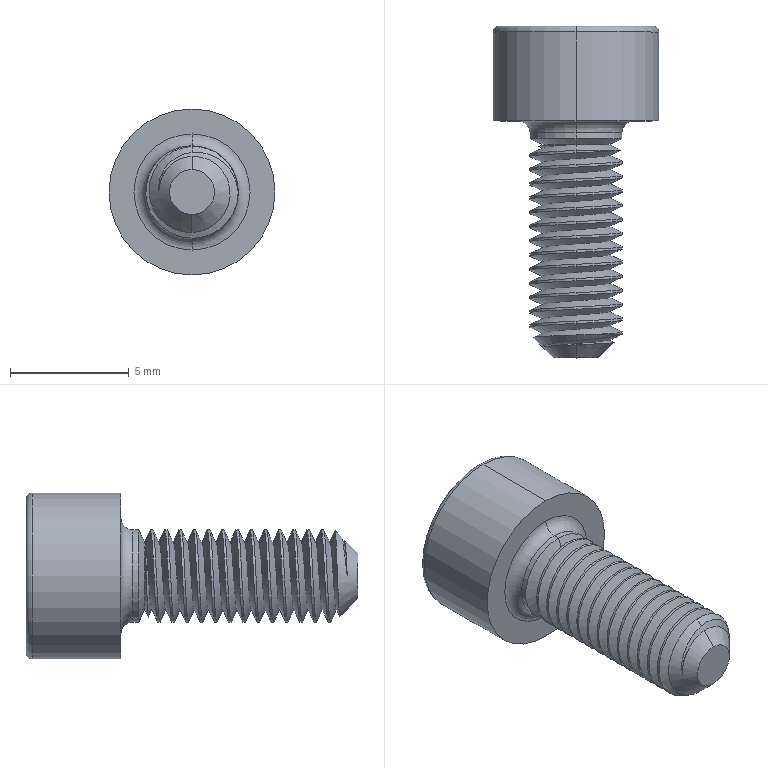Part | STEP file | Parafuso M4 - 10mm | 1 solid | 58 faces | box 7 x 14 x 7 mm | volume 220.851 mm3 | cylinder 31 | plane 10 | cone 9 | torus 6 | spline 2 | commonest cylinder face diameters 3.9 x29 7 x2